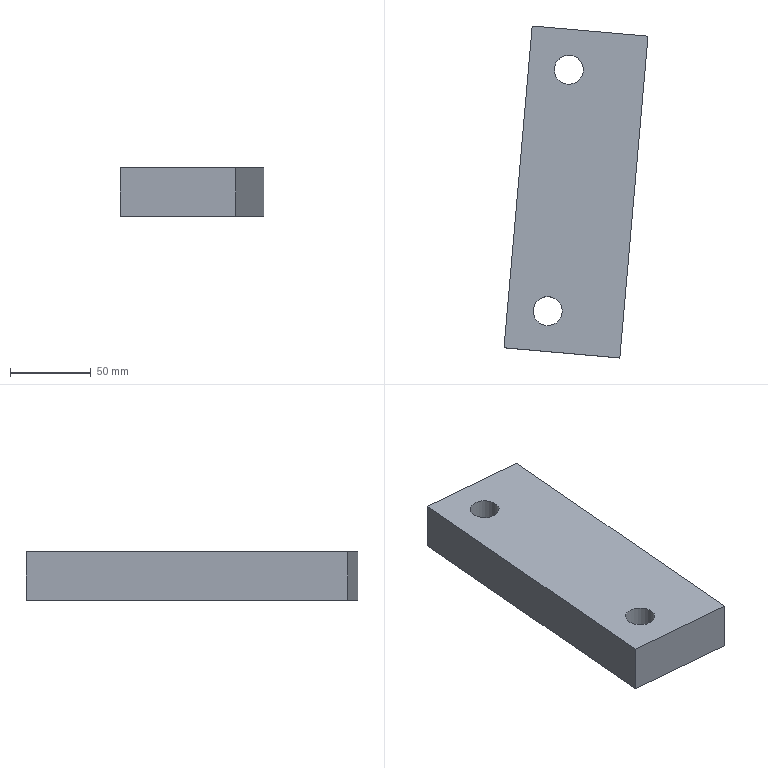Part | NX | features solid 2 | 1 solid | 8 faces | box 89.157 x 205.514 x 30 mm | volume 416732 mm3 | plane 6 | cylinder 2 | commonest cylinder face diameters 18 x2
STEP:
#1=CARTESIAN_POINT('',(175.983,-191.852,-70.));
#2=VERTEX_POINT('',#1);
#3=CARTESIAN_POINT('',(184.983,-191.852,-70.));
#4=DIRECTION('',(0.,0.,-1.));
#5=DIRECTION('',(-1.,0.,0.));
#6=AXIS2_PLACEMENT_3D('',#3,#4,#5);
#7=CIRCLE('',#6,9.);
#8=EDGE_CURVE('',#2,#2,#7,.T.);
#9=ORIENTED_EDGE('',*,*,#8,.F.);
#10=EDGE_LOOP('',(#9));
#11=FACE_BOUND('',#10,.T.);
#12=CARTESIAN_POINT('',(189.056,-42.423,-70.));
#13=VERTEX_POINT('',#12);
#14=CARTESIAN_POINT('',(198.056,-42.423,-70.));
#15=DIRECTION('',(0.,0.,-1.));
#16=DIRECTION('',(-1.,0.,0.));
#17=AXIS2_PLACEMENT_3D('',#14,#15,#16);
#18=CIRCLE('',#17,9.);
#19=EDGE_CURVE('',#13,#13,#18,.T.);
#20=ORIENTED_EDGE('',*,*,#19,.F.);
#21=EDGE_LOOP('',(#20));
#22=FACE_BOUND('',#21,.T.);
#23=CARTESIAN_POINT('',(157.899,-214.578,-70.));
#24=VERTEX_POINT('',#23);
#25=CARTESIAN_POINT('',(229.625,-220.854,-70.));
#26=VERTEX_POINT('',#25);
#27=CARTESIAN_POINT('',(196.751,-217.977,-70.));
#28=DIRECTION('',(-0.9962,0.08716,0.));
#29=VECTOR('',#28,1000.);
#30=LINE('',#27,#29);
#31=EDGE_CURVE('',#24,#26,#30,.F.);
#32=ORIENTED_EDGE('',*,*,#31,.F.);
#33=CARTESIAN_POINT('',(175.33,-15.339,-70.));
#34=VERTEX_POINT('',#33);
#35=CARTESIAN_POINT('',(162.257,-164.769,-70.));
#36=DIRECTION('',(-0.08716,-0.9962,0.));
#37=VECTOR('',#36,1000.);
#38=LINE('',#35,#37);
#39=EDGE_CURVE('',#24,#34,#38,.F.);
#40=ORIENTED_EDGE('',*,*,#39,.T.);
#41=CARTESIAN_POINT('',(247.056,-21.615,-70.));
#42=VERTEX_POINT('',#41);
#43=CARTESIAN_POINT('',(214.182,-18.738,-70.));
#44=DIRECTION('',(-0.9962,0.08716,0.));
#45=VECTOR('',#44,1000.);
#46=LINE('',#43,#45);
#47=EDGE_CURVE('',#34,#42,#46,.F.);
#48=ORIENTED_EDGE('',*,*,#47,.T.);
#49=CARTESIAN_POINT('',(233.983,-171.044,-70.));
#50=DIRECTION('',(0.08716,0.9962,0.));
#51=VECTOR('',#50,1000.);
#52=LINE('',#49,#51);
#53=EDGE_CURVE('',#26,#42,#52,.T.);
#54=ORIENTED_EDGE('',*,*,#53,.F.);
#55=EDGE_LOOP('',(#32,#40,#48,#54));
#56=FACE_BOUND('',#55,.T.);
#57=CARTESIAN_POINT('',(201.108,-168.168,-70.));
#58=DIRECTION('',(0.,0.,-1.));
#59=DIRECTION('',(0.08716,0.9962,0.));
#60=AXIS2_PLACEMENT_3D('',#57,#58,#59);
#61=PLANE('',#60);
#62=ADVANCED_FACE('',(#11,#22,#56),#61,.T.);
#63=ORIENTED_EDGE('',*,*,#47,.F.);
#64=CARTESIAN_POINT('',(175.33,-15.339,-40.));
#65=VERTEX_POINT('',#64);
#66=CARTESIAN_POINT('',(175.33,-15.339,-70.));
#67=DIRECTION('',(0.,0.,-1.));
#68=VECTOR('',#67,1000.);
#69=LINE('',#66,#68);
#70=EDGE_CURVE('',#34,#65,#69,.F.);
#71=ORIENTED_EDGE('',*,*,#70,.T.);
#72=CARTESIAN_POINT('',(247.056,-21.615,-40.));
#73=VERTEX_POINT('',#72);
#74=CARTESIAN_POINT('',(214.182,-18.738,-40.));
#75=DIRECTION('',(-0.9962,0.08716,0.));
#76=VECTOR('',#75,1000.);
#77=LINE('',#74,#76);
#78=EDGE_CURVE('',#65,#73,#77,.F.);
#79=ORIENTED_EDGE('',*,*,#78,.T.);
#80=CARTESIAN_POINT('',(247.056,-21.615,-70.));
#81=DIRECTION('',(0.,0.,1.));
#82=VECTOR('',#81,1000.);
#83=LINE('',#80,#82);
#84=EDGE_CURVE('',#42,#73,#83,.T.);
#85=ORIENTED_EDGE('',*,*,#84,.F.);
#86=EDGE_LOOP('',(#63,#71,#79,#85));
#87=FACE_BOUND('',#86,.T.);
#88=CARTESIAN_POINT('',(214.182,-18.738,-70.));
#89=DIRECTION('',(0.08716,0.9962,0.));
#90=DIRECTION('',(0.,0.,1.));
#91=AXIS2_PLACEMENT_3D('',#88,#89,#90);
#92=PLANE('',#91);
#93=ADVANCED_FACE('',(#87),#92,.T.);
#94=CARTESIAN_POINT('',(175.983,-191.852,-40.));
#95=VERTEX_POINT('',#94);
#96=CARTESIAN_POINT('',(184.983,-191.852,-40.));
#97=DIRECTION('',(0.,0.,-1.));
#98=DIRECTION('',(-1.,0.,0.));
#99=AXIS2_PLACEMENT_3D('',#96,#97,#98);
#100=CIRCLE('',#99,9.);
#101=EDGE_CURVE('',#95,#95,#100,.F.);
#102=ORIENTED_EDGE('',*,*,#101,.F.);
#103=EDGE_LOOP('',(#102));
#104=FACE_BOUND('',#103,.T.);
#105=CARTESIAN_POINT('',(189.056,-42.423,-40.));
#106=VERTEX_POINT('',#105);
#107=CARTESIAN_POINT('',(198.056,-42.423,-40.));
#108=DIRECTION('',(0.,0.,-1.));
#109=DIRECTION('',(-1.,0.,0.));
#110=AXIS2_PLACEMENT_3D('',#107,#108,#109);
#111=CIRCLE('',#110,9.);
#112=EDGE_CURVE('',#106,#106,#111,.F.);
#113=ORIENTED_EDGE('',*,*,#112,.F.);
#114=EDGE_LOOP('',(#113));
#115=FACE_BOUND('',#114,.T.);
#116=ORIENTED_EDGE('',*,*,#78,.F.);
#117=CARTESIAN_POINT('',(157.899,-214.578,-40.));
#118=VERTEX_POINT('',#117);
#119=CARTESIAN_POINT('',(162.257,-164.769,-40.));
#120=DIRECTION('',(0.08716,0.9962,0.));
#121=VECTOR('',#120,1000.);
#122=LINE('',#119,#121);
#123=EDGE_CURVE('',#118,#65,#122,.T.);
#124=ORIENTED_EDGE('',*,*,#123,.F.);
#125=CARTESIAN_POINT('',(229.625,-220.854,-40.));
#126=VERTEX_POINT('',#125);
#127=CARTESIAN_POINT('',(196.751,-217.977,-40.));
#128=DIRECTION('',(0.9962,-0.08716,0.));
#129=VECTOR('',#128,1000.);
#130=LINE('',#127,#129);
#131=EDGE_CURVE('',#118,#126,#130,.T.);
#132=ORIENTED_EDGE('',*,*,#131,.T.);
#133=CARTESIAN_POINT('',(233.983,-171.044,-40.));
#134=DIRECTION('',(0.08716,0.9962,0.));
#135=VECTOR('',#134,1000.);
#136=LINE('',#133,#135);
#137=EDGE_CURVE('',#126,#73,#136,.T.);
#138=ORIENTED_EDGE('',*,*,#137,.T.);
#139=EDGE_LOOP('',(#116,#124,#132,#138));
#140=FACE_BOUND('',#139,.T.);
#141=CARTESIAN_POINT('',(201.108,-168.168,-40.));
#142=DIRECTION('',(0.,0.,-1.));
#143=DIRECTION('',(0.08716,0.9962,0.));
#144=AXIS2_PLACEMENT_3D('',#141,#142,#143);
#145=PLANE('',#144);
#146=ADVANCED_FACE('',(#104,#115,#140),#145,.F.);
#147=CARTESIAN_POINT('',(157.899,-214.578,-70.));
#148=DIRECTION('',(0.,0.,1.));
#149=VECTOR('',#148,1000.);
#150=LINE('',#147,#149);
#151=EDGE_CURVE('',#24,#118,#150,.T.);
#152=ORIENTED_EDGE('',*,*,#151,.F.);
#153=ORIENTED_EDGE('',*,*,#31,.T.);
#154=CARTESIAN_POINT('',(229.625,-220.854,-70.));
#155=DIRECTION('',(0.,0.,1.));
#156=VECTOR('',#155,1000.);
#157=LINE('',#154,#156);
#158=EDGE_CURVE('',#26,#126,#157,.T.);
#159=ORIENTED_EDGE('',*,*,#158,.T.);
#160=ORIENTED_EDGE('',*,*,#131,.F.);
#161=EDGE_LOOP('',(#152,#153,#159,#160));
#162=FACE_BOUND('',#161,.T.);
#163=CARTESIAN_POINT('',(196.751,-217.977,-70.));
#164=DIRECTION('',(0.08716,0.9962,0.));
#165=DIRECTION('',(0.,0.,1.));
#166=AXIS2_PLACEMENT_3D('',#163,#164,#165);
#167=PLANE('',#166);
#168=ADVANCED_FACE('',(#162),#167,.F.);
#169=ORIENTED_EDGE('',*,*,#137,.F.);
#170=ORIENTED_EDGE('',*,*,#158,.F.);
#171=ORIENTED_EDGE('',*,*,#53,.T.);
#172=ORIENTED_EDGE('',*,*,#84,.T.);
#173=EDGE_LOOP('',(#169,#170,#171,#172));
#174=FACE_BOUND('',#173,.T.);
#175=CARTESIAN_POINT('',(233.983,-171.044,-70.));
#176=DIRECTION('',(-0.9962,0.08716,0.));
#177=DIRECTION('',(0.08716,0.9962,0.));
#178=AXIS2_PLACEMENT_3D('',#175,#176,#177);
#179=PLANE('',#178);
#180=ADVANCED_FACE('',(#174),#179,.F.);
#181=ORIENTED_EDGE('',*,*,#123,.T.);
#182=ORIENTED_EDGE('',*,*,#70,.F.);
#183=ORIENTED_EDGE('',*,*,#39,.F.);
#184=ORIENTED_EDGE('',*,*,#151,.T.);
#185=EDGE_LOOP('',(#181,#182,#183,#184));
#186=FACE_BOUND('',#185,.T.);
#187=CARTESIAN_POINT('',(162.257,-164.769,-70.));
#188=DIRECTION('',(-0.9962,0.08716,0.));
#189=DIRECTION('',(0.08716,0.9962,0.));
#190=AXIS2_PLACEMENT_3D('',#187,#188,#189);
#191=PLANE('',#190);
#192=ADVANCED_FACE('',(#186),#191,.T.);
#193=ORIENTED_EDGE('',*,*,#112,.T.);
#194=EDGE_LOOP('',(#193));
#195=FACE_BOUND('',#194,.T.);
#196=ORIENTED_EDGE('',*,*,#19,.T.);
#197=EDGE_LOOP('',(#196));
#198=FACE_BOUND('',#197,.T.);
#199=CARTESIAN_POINT('',(198.056,-42.423,-195.));
#200=DIRECTION('',(0.,0.,1.));
#201=DIRECTION('',(0.9848,-0.1736,0.));
#202=AXIS2_PLACEMENT_3D('',#199,#200,#201);
#203=CYLINDRICAL_SURFACE('',#202,9.);
#204=ADVANCED_FACE('',(#195,#198),#203,.F.);
#205=ORIENTED_EDGE('',*,*,#101,.T.);
#206=EDGE_LOOP('',(#205));
#207=FACE_BOUND('',#206,.T.);
#208=ORIENTED_EDGE('',*,*,#8,.T.);
#209=EDGE_LOOP('',(#208));
#210=FACE_BOUND('',#209,.T.);
#211=CARTESIAN_POINT('',(184.983,-191.852,-195.));
#212=DIRECTION('',(0.,0.,1.));
#213=DIRECTION('',(0.9848,-0.1736,0.));
#214=AXIS2_PLACEMENT_3D('',#211,#212,#213);
#215=CYLINDRICAL_SURFACE('',#214,9.);
#216=ADVANCED_FACE('',(#207,#210),#215,.F.);
#217=CLOSED_SHELL('',(#62,#93,#146,#168,#180,#192,#204,#216));
#218=MANIFOLD_SOLID_BREP('',#217);
#219=(LENGTH_UNIT()NAMED_UNIT(*)SI_UNIT(.MILLI.,.METRE.));
#220=UNCERTAINTY_MEASURE_WITH_UNIT(LENGTH_MEASURE(0.00001),#219,'','');
#221=(NAMED_UNIT(*)PLANE_ANGLE_UNIT()SI_UNIT($,.RADIAN.));
#222=(NAMED_UNIT(*)SI_UNIT($,.STERADIAN.)SOLID_ANGLE_UNIT());
#223=(GEOMETRIC_REPRESENTATION_CONTEXT(3)GLOBAL_UNCERTAINTY_ASSIGNED_CONTEXT((#220))GLOBAL_UNIT_ASSIGNED_CONTEXT((#219,#221,#222))REPRESENTATION_CONTEXT('',''));
#224=ADVANCED_BREP_SHAPE_REPRESENTATION('',(#218),#223);